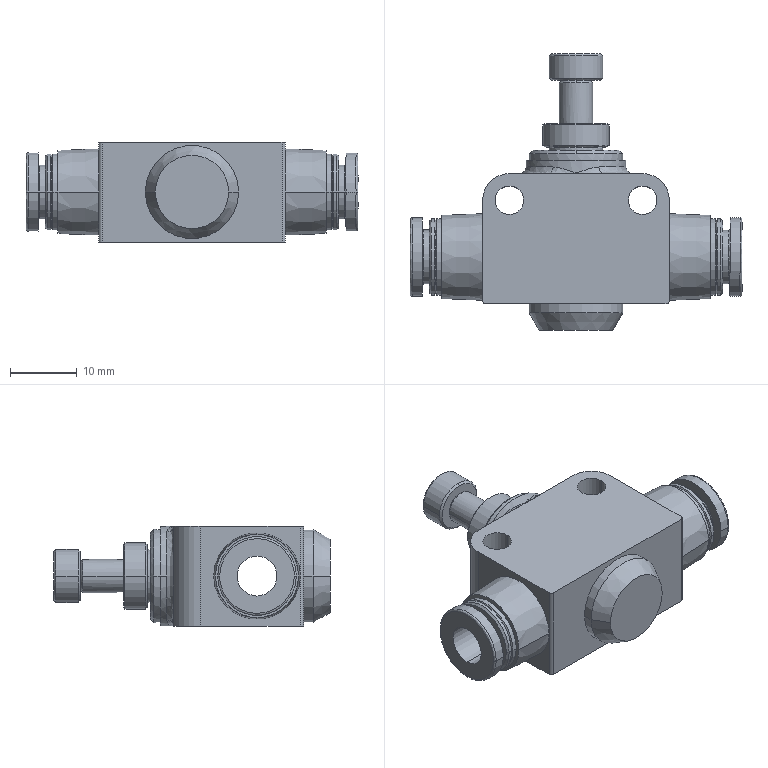Part | STEP file | 0246_014_SPJYS6 | 1 solid | 110 faces | box 49.8 x 41.5 x 15 mm | volume 10430 mm3 | cylinder 40 | cone 36 | plane 22 | spline 12 | commonest cylinder face diameters 11.48 x8 4.3 x4 7.98 x4 1 x2 4.98 x2 6 x2